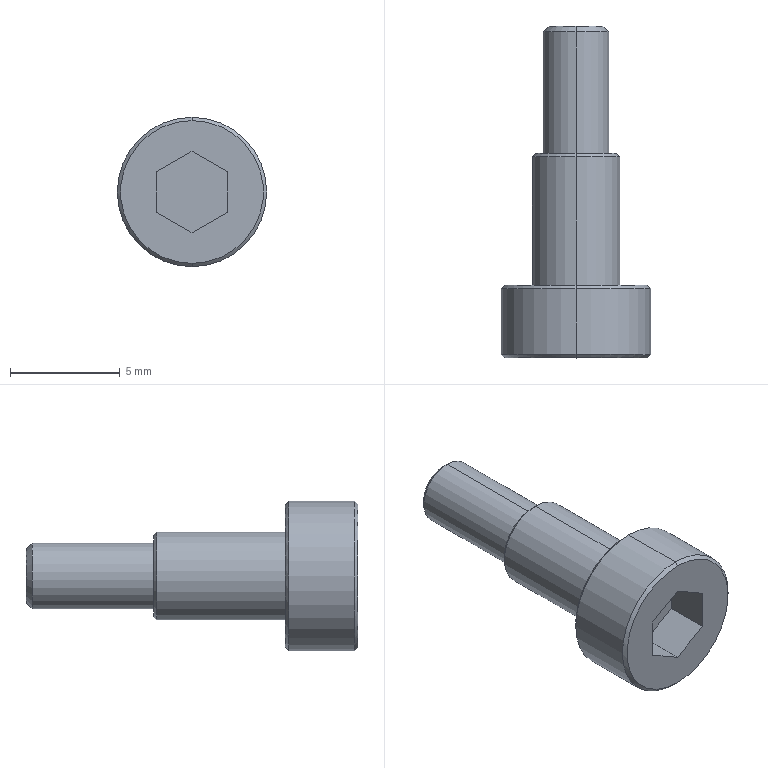Part | SolidWorks | features ICE 2, Chamfer 1, Extrusion 1, StudWizard 1 | 1 solid | 25 faces | box 6.8 x 15.1 x 6.8 mm | volume 217.57 mm3 | plane 11 | cone 8 | cylinder 6 | commonest cylinder face diameters 3 x2 4 x2 6.8 x2
STEP:
#1=CARTESIAN_POINT('',(0.,9.3,1.85));
#2=VERTEX_POINT('',#1);
#3=CARTESIAN_POINT('',(0.,9.3,-1.85));
#4=VERTEX_POINT('',#3);
#5=CARTESIAN_POINT('',(0.,9.3,0.));
#6=DIRECTION('',(0.,1.,0.));
#7=DIRECTION('',(0.,0.,1.));
#8=AXIS2_PLACEMENT_3D('',#5,#6,#7);
#9=CIRCLE('',#8,1.85);
#10=EDGE_CURVE('',#2,#4,#9,.T.);
#11=ORIENTED_EDGE('',*,*,#10,.F.);
#12=CARTESIAN_POINT('',(0.,9.15,2.));
#13=VERTEX_POINT('',#12);
#14=CARTESIAN_POINT('',(0.,9.3,1.85));
#15=DIRECTION('',(0.,-0.7071,0.7071));
#16=VECTOR('',#15,1000.);
#17=LINE('',#14,#16);
#18=EDGE_CURVE('',#2,#13,#17,.T.);
#19=ORIENTED_EDGE('',*,*,#18,.T.);
#20=CARTESIAN_POINT('',(0.,9.15,-2.));
#21=VERTEX_POINT('',#20);
#22=CARTESIAN_POINT('',(0.,9.15,0.));
#23=DIRECTION('',(0.,-1.,0.));
#24=DIRECTION('',(0.,0.,1.));
#25=AXIS2_PLACEMENT_3D('',#22,#23,#24);
#26=CIRCLE('',#25,2.);
#27=EDGE_CURVE('',#21,#13,#26,.T.);
#28=ORIENTED_EDGE('',*,*,#27,.F.);
#29=CARTESIAN_POINT('',(0.,9.3,-1.85));
#30=DIRECTION('',(0.,-0.7071,-0.7071));
#31=VECTOR('',#30,1000.);
#32=LINE('',#29,#31);
#33=EDGE_CURVE('',#4,#21,#32,.T.);
#34=ORIENTED_EDGE('',*,*,#33,.F.);
#35=EDGE_LOOP('',(#11,#19,#28,#34));
#36=FACE_OUTER_BOUND('',#35,.T.);
#37=CARTESIAN_POINT('',(0.,9.3,0.));
#38=DIRECTION('',(0.,-1.,0.));
#39=DIRECTION('',(0.,0.,-1.));
#40=AXIS2_PLACEMENT_3D('',#37,#38,#39);
#41=CONICAL_SURFACE('',#40,1.85,0.7854);
#42=ADVANCED_FACE('',(#36),#41,.T.);
#43=CARTESIAN_POINT('',(0.,3.3,3.25));
#44=VERTEX_POINT('',#43);
#45=CARTESIAN_POINT('',(0.,3.3,-3.25));
#46=VERTEX_POINT('',#45);
#47=CARTESIAN_POINT('',(0.,3.3,0.));
#48=DIRECTION('',(0.,1.,0.));
#49=DIRECTION('',(0.,0.,1.));
#50=AXIS2_PLACEMENT_3D('',#47,#48,#49);
#51=CIRCLE('',#50,3.25);
#52=EDGE_CURVE('',#44,#46,#51,.T.);
#53=ORIENTED_EDGE('',*,*,#52,.F.);
#54=CARTESIAN_POINT('',(0.,3.15,3.4));
#55=VERTEX_POINT('',#54);
#56=CARTESIAN_POINT('',(0.,3.3,3.25));
#57=DIRECTION('',(0.,-0.7071,0.7071));
#58=VECTOR('',#57,1000.);
#59=LINE('',#56,#58);
#60=EDGE_CURVE('',#44,#55,#59,.T.);
#61=ORIENTED_EDGE('',*,*,#60,.T.);
#62=CARTESIAN_POINT('',(0.,3.15,-3.4));
#63=VERTEX_POINT('',#62);
#64=CARTESIAN_POINT('',(0.,3.15,0.));
#65=DIRECTION('',(0.,-1.,0.));
#66=DIRECTION('',(0.,0.,1.));
#67=AXIS2_PLACEMENT_3D('',#64,#65,#66);
#68=CIRCLE('',#67,3.4);
#69=EDGE_CURVE('',#63,#55,#68,.T.);
#70=ORIENTED_EDGE('',*,*,#69,.F.);
#71=CARTESIAN_POINT('',(0.,3.3,-3.25));
#72=DIRECTION('',(0.,-0.7071,-0.7071));
#73=VECTOR('',#72,1000.);
#74=LINE('',#71,#73);
#75=EDGE_CURVE('',#46,#63,#74,.T.);
#76=ORIENTED_EDGE('',*,*,#75,.F.);
#77=EDGE_LOOP('',(#53,#61,#70,#76));
#78=FACE_OUTER_BOUND('',#77,.T.);
#79=CARTESIAN_POINT('',(0.,3.3,0.));
#80=DIRECTION('',(0.,-1.,0.));
#81=DIRECTION('',(0.,0.,-1.));
#82=AXIS2_PLACEMENT_3D('',#79,#80,#81);
#83=CONICAL_SURFACE('',#82,3.25,0.7854);
#84=ADVANCED_FACE('',(#78),#83,.T.);
#85=CARTESIAN_POINT('',(0.,0.,-3.25));
#86=VERTEX_POINT('',#85);
#87=CARTESIAN_POINT('',(0.,0.,3.25));
#88=VERTEX_POINT('',#87);
#89=CARTESIAN_POINT('',(0.,0.,0.));
#90=DIRECTION('',(0.,-1.,0.));
#91=DIRECTION('',(0.,0.,1.));
#92=AXIS2_PLACEMENT_3D('',#89,#90,#91);
#93=CIRCLE('',#92,3.25);
#94=EDGE_CURVE('',#86,#88,#93,.T.);
#95=ORIENTED_EDGE('',*,*,#94,.F.);
#96=CARTESIAN_POINT('',(0.,0.15,-3.4));
#97=VERTEX_POINT('',#96);
#98=CARTESIAN_POINT('',(0.,0.15,-3.4));
#99=DIRECTION('',(0.,0.7071,-0.7071));
#100=VECTOR('',#99,1000.);
#101=LINE('',#98,#100);
#102=EDGE_CURVE('',#86,#97,#101,.T.);
#103=ORIENTED_EDGE('',*,*,#102,.T.);
#104=CARTESIAN_POINT('',(0.,0.15,3.4));
#105=VERTEX_POINT('',#104);
#106=CARTESIAN_POINT('',(0.,0.15,0.));
#107=DIRECTION('',(0.,1.,0.));
#108=DIRECTION('',(0.,0.,1.));
#109=AXIS2_PLACEMENT_3D('',#106,#107,#108);
#110=CIRCLE('',#109,3.4);
#111=EDGE_CURVE('',#105,#97,#110,.T.);
#112=ORIENTED_EDGE('',*,*,#111,.F.);
#113=CARTESIAN_POINT('',(0.,0.15,3.4));
#114=DIRECTION('',(0.,0.7071,0.7071));
#115=VECTOR('',#114,1000.);
#116=LINE('',#113,#115);
#117=EDGE_CURVE('',#88,#105,#116,.T.);
#118=ORIENTED_EDGE('',*,*,#117,.F.);
#119=EDGE_LOOP('',(#95,#103,#112,#118));
#120=FACE_OUTER_BOUND('',#119,.T.);
#121=CARTESIAN_POINT('',(0.,0.15,0.));
#122=DIRECTION('',(0.,1.,0.));
#123=DIRECTION('',(0.,0.,1.));
#124=AXIS2_PLACEMENT_3D('',#121,#122,#123);
#125=CONICAL_SURFACE('',#124,3.4,0.7854);
#126=ADVANCED_FACE('',(#120),#125,.T.);
#127=CARTESIAN_POINT('',(0.,14.83,-1.5));
#128=VERTEX_POINT('',#127);
#129=CARTESIAN_POINT('',(0.,14.83,1.5));
#130=VERTEX_POINT('',#129);
#131=CARTESIAN_POINT('',(0.,14.83,0.));
#132=DIRECTION('',(0.,-1.,0.));
#133=DIRECTION('',(0.,0.,-1.));
#134=AXIS2_PLACEMENT_3D('',#131,#132,#133);
#135=CIRCLE('',#134,1.5);
#136=EDGE_CURVE('',#128,#130,#135,.T.);
#137=ORIENTED_EDGE('',*,*,#136,.T.);
#138=CARTESIAN_POINT('',(0.,9.3,1.5));
#139=VERTEX_POINT('',#138);
#140=CARTESIAN_POINT('',(0.,9.3,1.5));
#141=DIRECTION('',(0.,-1.,0.));
#142=VECTOR('',#141,1000.);
#143=LINE('',#140,#142);
#144=EDGE_CURVE('',#130,#139,#143,.T.);
#145=ORIENTED_EDGE('',*,*,#144,.T.);
#146=CARTESIAN_POINT('',(0.,9.3,-1.5));
#147=VERTEX_POINT('',#146);
#148=CARTESIAN_POINT('',(0.,9.3,0.));
#149=DIRECTION('',(0.,-1.,0.));
#150=DIRECTION('',(0.,0.,-1.));
#151=AXIS2_PLACEMENT_3D('',#148,#149,#150);
#152=CIRCLE('',#151,1.5);
#153=EDGE_CURVE('',#147,#139,#152,.T.);
#154=ORIENTED_EDGE('',*,*,#153,.F.);
#155=CARTESIAN_POINT('',(0.,9.3,-1.5));
#156=DIRECTION('',(0.,-1.,0.));
#157=VECTOR('',#156,1000.);
#158=LINE('',#155,#157);
#159=EDGE_CURVE('',#128,#147,#158,.T.);
#160=ORIENTED_EDGE('',*,*,#159,.F.);
#161=EDGE_LOOP('',(#137,#145,#154,#160));
#162=FACE_OUTER_BOUND('',#161,.T.);
#163=CARTESIAN_POINT('',(0.,9.3,0.));
#164=DIRECTION('',(0.,-1.,0.));
#165=DIRECTION('',(0.,0.,-1.));
#166=AXIS2_PLACEMENT_3D('',#163,#164,#165);
#167=CYLINDRICAL_SURFACE('',#166,1.5);
#168=ADVANCED_FACE('',(#162),#167,.T.);
#169=CARTESIAN_POINT('',(0.,15.1,-1.23));
#170=VERTEX_POINT('',#169);
#171=CARTESIAN_POINT('',(0.,15.1,1.23));
#172=VERTEX_POINT('',#171);
#173=CARTESIAN_POINT('',(0.,15.1,0.));
#174=DIRECTION('',(0.,-1.,0.));
#175=DIRECTION('',(0.,0.,-1.));
#176=AXIS2_PLACEMENT_3D('',#173,#174,#175);
#177=CIRCLE('',#176,1.23);
#178=EDGE_CURVE('',#170,#172,#177,.T.);
#179=ORIENTED_EDGE('',*,*,#178,.T.);
#180=CARTESIAN_POINT('',(0.,14.83,1.5));
#181=DIRECTION('',(0.,-0.7071,0.7071));
#182=VECTOR('',#181,1000.);
#183=LINE('',#180,#182);
#184=EDGE_CURVE('',#172,#130,#183,.T.);
#185=ORIENTED_EDGE('',*,*,#184,.T.);
#186=ORIENTED_EDGE('',*,*,#136,.F.);
#187=CARTESIAN_POINT('',(0.,14.83,-1.5));
#188=DIRECTION('',(0.,-0.7071,-0.7071));
#189=VECTOR('',#188,1000.);
#190=LINE('',#187,#189);
#191=EDGE_CURVE('',#170,#128,#190,.T.);
#192=ORIENTED_EDGE('',*,*,#191,.F.);
#193=EDGE_LOOP('',(#179,#185,#186,#192));
#194=FACE_OUTER_BOUND('',#193,.T.);
#195=CARTESIAN_POINT('',(0.,14.83,0.));
#196=DIRECTION('',(0.,-1.,0.));
#197=DIRECTION('',(0.,0.,-1.));
#198=AXIS2_PLACEMENT_3D('',#195,#196,#197);
#199=CONICAL_SURFACE('',#198,1.5,0.7854);
#200=ADVANCED_FACE('',(#194),#199,.T.);
#201=ORIENTED_EDGE('',*,*,#27,.T.);
#202=CARTESIAN_POINT('',(0.,3.3,2.));
#203=VERTEX_POINT('',#202);
#204=CARTESIAN_POINT('',(0.,9.3,2.));
#205=DIRECTION('',(0.,-1.,0.));
#206=VECTOR('',#205,1000.);
#207=LINE('',#204,#206);
#208=EDGE_CURVE('',#13,#203,#207,.T.);
#209=ORIENTED_EDGE('',*,*,#208,.T.);
#210=CARTESIAN_POINT('',(0.,3.3,-2.));
#211=VERTEX_POINT('',#210);
#212=CARTESIAN_POINT('',(0.,3.3,0.));
#213=DIRECTION('',(0.,1.,0.));
#214=DIRECTION('',(0.,0.,1.));
#215=AXIS2_PLACEMENT_3D('',#212,#213,#214);
#216=CIRCLE('',#215,2.);
#217=EDGE_CURVE('',#203,#211,#216,.T.);
#218=ORIENTED_EDGE('',*,*,#217,.T.);
#219=CARTESIAN_POINT('',(0.,9.3,-2.));
#220=DIRECTION('',(0.,-1.,0.));
#221=VECTOR('',#220,1000.);
#222=LINE('',#219,#221);
#223=EDGE_CURVE('',#21,#211,#222,.T.);
#224=ORIENTED_EDGE('',*,*,#223,.F.);
#225=EDGE_LOOP('',(#201,#209,#218,#224));
#226=FACE_OUTER_BOUND('',#225,.T.);
#227=CARTESIAN_POINT('',(0.,9.3,0.));
#228=DIRECTION('',(0.,-1.,0.));
#229=DIRECTION('',(0.,0.,-1.));
#230=AXIS2_PLACEMENT_3D('',#227,#228,#229);
#231=CYLINDRICAL_SURFACE('',#230,2.);
#232=ADVANCED_FACE('',(#226),#231,.T.);
#233=ORIENTED_EDGE('',*,*,#69,.T.);
#234=CARTESIAN_POINT('',(0.,3.3,3.4));
#235=DIRECTION('',(0.,-1.,0.));
#236=VECTOR('',#235,1000.);
#237=LINE('',#234,#236);
#238=EDGE_CURVE('',#55,#105,#237,.T.);
#239=ORIENTED_EDGE('',*,*,#238,.T.);
#240=ORIENTED_EDGE('',*,*,#111,.T.);
#241=CARTESIAN_POINT('',(0.,3.3,-3.4));
#242=DIRECTION('',(0.,-1.,0.));
#243=VECTOR('',#242,1000.);
#244=LINE('',#241,#243);
#245=EDGE_CURVE('',#63,#97,#244,.T.);
#246=ORIENTED_EDGE('',*,*,#245,.F.);
#247=EDGE_LOOP('',(#233,#239,#240,#246));
#248=FACE_OUTER_BOUND('',#247,.T.);
#249=CARTESIAN_POINT('',(0.,3.3,0.));
#250=DIRECTION('',(0.,-1.,0.));
#251=DIRECTION('',(0.,0.,-1.));
#252=AXIS2_PLACEMENT_3D('',#249,#250,#251);
#253=CYLINDRICAL_SURFACE('',#252,3.4);
#254=ADVANCED_FACE('',(#248),#253,.T.);
#255=ORIENTED_EDGE('',*,*,#238,.F.);
#256=CARTESIAN_POINT('',(0.,3.15,0.));
#257=DIRECTION('',(0.,-1.,0.));
#258=DIRECTION('',(0.,0.,1.));
#259=AXIS2_PLACEMENT_3D('',#256,#257,#258);
#260=CIRCLE('',#259,3.4);
#261=EDGE_CURVE('',#55,#63,#260,.T.);
#262=ORIENTED_EDGE('',*,*,#261,.T.);
#263=ORIENTED_EDGE('',*,*,#245,.T.);
#264=CARTESIAN_POINT('',(0.,0.15,0.));
#265=DIRECTION('',(0.,1.,0.));
#266=DIRECTION('',(0.,0.,1.));
#267=AXIS2_PLACEMENT_3D('',#264,#265,#266);
#268=CIRCLE('',#267,3.4);
#269=EDGE_CURVE('',#97,#105,#268,.T.);
#270=ORIENTED_EDGE('',*,*,#269,.T.);
#271=EDGE_LOOP('',(#255,#262,#263,#270));
#272=FACE_OUTER_BOUND('',#271,.T.);
#273=CARTESIAN_POINT('',(0.,3.3,0.));
#274=DIRECTION('',(0.,-1.,0.));
#275=DIRECTION('',(0.,0.,-1.));
#276=AXIS2_PLACEMENT_3D('',#273,#274,#275);
#277=CYLINDRICAL_SURFACE('',#276,3.4);
#278=ADVANCED_FACE('',(#272),#277,.T.);
#279=CARTESIAN_POINT('',(0.,3.3,0.));
#280=DIRECTION('',(0.,1.,0.));
#281=DIRECTION('',(0.,0.,1.));
#282=AXIS2_PLACEMENT_3D('',#279,#280,#281);
#283=CIRCLE('',#282,3.25);
#284=EDGE_CURVE('',#46,#44,#283,.T.);
#285=ORIENTED_EDGE('',*,*,#284,.T.);
#286=ORIENTED_EDGE('',*,*,#52,.T.);
#287=EDGE_LOOP('',(#285,#286));
#288=FACE_OUTER_BOUND('',#287,.T.);
#289=CARTESIAN_POINT('',(0.,3.3,0.));
#290=DIRECTION('',(0.,1.,0.));
#291=DIRECTION('',(0.,0.,1.));
#292=AXIS2_PLACEMENT_3D('',#289,#290,#291);
#293=CIRCLE('',#292,2.);
#294=EDGE_CURVE('',#211,#203,#293,.T.);
#295=ORIENTED_EDGE('',*,*,#294,.F.);
#296=ORIENTED_EDGE('',*,*,#217,.F.);
#297=EDGE_LOOP('',(#295,#296));
#298=FACE_BOUND('',#297,.T.);
#299=CARTESIAN_POINT('',(0.,3.3,0.));
#300=DIRECTION('',(0.,1.,0.));
#301=DIRECTION('',(0.,0.,1.));
#302=AXIS2_PLACEMENT_3D('',#299,#300,#301);
#303=PLANE('',#302);
#304=ADVANCED_FACE('',(#288,#298),#303,.T.);
#305=CARTESIAN_POINT('',(0.,0.,0.));
#306=DIRECTION('',(0.,-1.,0.));
#307=DIRECTION('',(0.,0.,1.));
#308=AXIS2_PLACEMENT_3D('',#305,#306,#307);
#309=CIRCLE('',#308,3.25);
#310=EDGE_CURVE('',#88,#86,#309,.T.);
#311=ORIENTED_EDGE('',*,*,#310,.T.);
#312=ORIENTED_EDGE('',*,*,#94,.T.);
#313=EDGE_LOOP('',(#311,#312));
#314=FACE_OUTER_BOUND('',#313,.T.);
#315=CARTESIAN_POINT('',(0.,0.,1.848));
#316=VERTEX_POINT('',#315);
#317=CARTESIAN_POINT('',(-1.6,0.,0.9238));
#318=VERTEX_POINT('',#317);
#319=CARTESIAN_POINT('',(0.,0.,1.848));
#320=DIRECTION('',(-0.866,0.,-0.5));
#321=VECTOR('',#320,1000.);
#322=LINE('',#319,#321);
#323=EDGE_CURVE('',#316,#318,#322,.T.);
#324=ORIENTED_EDGE('',*,*,#323,.F.);
#325=CARTESIAN_POINT('',(1.6,0.,0.9238));
#326=VERTEX_POINT('',#325);
#327=CARTESIAN_POINT('',(1.6,0.,0.9238));
#328=DIRECTION('',(-0.866,0.,0.5));
#329=VECTOR('',#328,1000.);
#330=LINE('',#327,#329);
#331=EDGE_CURVE('',#326,#316,#330,.T.);
#332=ORIENTED_EDGE('',*,*,#331,.F.);
#333=CARTESIAN_POINT('',(1.6,0.,-0.9238));
#334=VERTEX_POINT('',#333);
#335=CARTESIAN_POINT('',(1.6,0.,-0.9238));
#336=DIRECTION('',(0.,0.,1.));
#337=VECTOR('',#336,1000.);
#338=LINE('',#335,#337);
#339=EDGE_CURVE('',#334,#326,#338,.T.);
#340=ORIENTED_EDGE('',*,*,#339,.F.);
#341=CARTESIAN_POINT('',(0.,0.,-1.848));
#342=VERTEX_POINT('',#341);
#343=CARTESIAN_POINT('',(0.,0.,-1.848));
#344=DIRECTION('',(0.866,0.,0.5));
#345=VECTOR('',#344,1000.);
#346=LINE('',#343,#345);
#347=EDGE_CURVE('',#342,#334,#346,.T.);
#348=ORIENTED_EDGE('',*,*,#347,.F.);
#349=CARTESIAN_POINT('',(-1.6,0.,-0.9238));
#350=VERTEX_POINT('',#349);
#351=CARTESIAN_POINT('',(-1.6,0.,-0.9238));
#352=DIRECTION('',(0.866,0.,-0.5));
#353=VECTOR('',#352,1000.);
#354=LINE('',#351,#353);
#355=EDGE_CURVE('',#350,#342,#354,.T.);
#356=ORIENTED_EDGE('',*,*,#355,.F.);
#357=CARTESIAN_POINT('',(-1.6,0.,0.9238));
#358=DIRECTION('',(0.,0.,-1.));
#359=VECTOR('',#358,1000.);
#360=LINE('',#357,#359);
#361=EDGE_CURVE('',#318,#350,#360,.T.);
#362=ORIENTED_EDGE('',*,*,#361,.F.);
#363=EDGE_LOOP('',(#324,#332,#340,#348,#356,#362));
#364=FACE_BOUND('',#363,.T.);
#365=CARTESIAN_POINT('',(0.,0.,0.));
#366=DIRECTION('',(0.,1.,0.));
#367=DIRECTION('',(0.,0.,1.));
#368=AXIS2_PLACEMENT_3D('',#365,#366,#367);
#369=PLANE('',#368);
#370=ADVANCED_FACE('',(#314,#364),#369,.F.);
#371=ORIENTED_EDGE('',*,*,#208,.F.);
#372=CARTESIAN_POINT('',(0.,9.15,0.));
#373=DIRECTION('',(0.,-1.,0.));
#374=DIRECTION('',(0.,0.,1.));
#375=AXIS2_PLACEMENT_3D('',#372,#373,#374);
#376=CIRCLE('',#375,2.);
#377=EDGE_CURVE('',#13,#21,#376,.T.);
#378=ORIENTED_EDGE('',*,*,#377,.T.);
#379=ORIENTED_EDGE('',*,*,#223,.T.);
#380=ORIENTED_EDGE('',*,*,#294,.T.);
#381=EDGE_LOOP('',(#371,#378,#379,#380));
#382=FACE_OUTER_BOUND('',#381,.T.);
#383=CARTESIAN_POINT('',(0.,9.3,0.));
#384=DIRECTION('',(0.,-1.,0.));
#385=DIRECTION('',(0.,0.,-1.));
#386=AXIS2_PLACEMENT_3D('',#383,#384,#385);
#387=CYLINDRICAL_SURFACE('',#386,2.);
#388=ADVANCED_FACE('',(#382),#387,.T.);
#389=CARTESIAN_POINT('',(0.,9.3,0.));
#390=DIRECTION('',(0.,1.,0.));
#391=DIRECTION('',(0.,0.,1.));
#392=AXIS2_PLACEMENT_3D('',#389,#390,#391);
#393=CIRCLE('',#392,1.85);
#394=EDGE_CURVE('',#4,#2,#393,.T.);
#395=ORIENTED_EDGE('',*,*,#394,.T.);
#396=ORIENTED_EDGE('',*,*,#10,.T.);
#397=EDGE_LOOP('',(#395,#396));
#398=FACE_OUTER_BOUND('',#397,.T.);
#399=ORIENTED_EDGE('',*,*,#153,.T.);
#400=CARTESIAN_POINT('',(0.,9.3,0.));
#401=DIRECTION('',(0.,-1.,0.));
#402=DIRECTION('',(0.,0.,-1.));
#403=AXIS2_PLACEMENT_3D('',#400,#401,#402);
#404=CIRCLE('',#403,1.5);
#405=EDGE_CURVE('',#139,#147,#404,.T.);
#406=ORIENTED_EDGE('',*,*,#405,.T.);
#407=EDGE_LOOP('',(#399,#406));
#408=FACE_BOUND('',#407,.T.);
#409=CARTESIAN_POINT('',(0.,9.3,0.));
#410=DIRECTION('',(0.,1.,0.));
#411=DIRECTION('',(0.,0.,1.));
#412=AXIS2_PLACEMENT_3D('',#409,#410,#411);
#413=PLANE('',#412);
#414=ADVANCED_FACE('',(#398,#408),#413,.T.);
#415=ORIENTED_EDGE('',*,*,#178,.F.);
#416=CARTESIAN_POINT('',(0.,15.1,0.));
#417=DIRECTION('',(0.,-1.,0.));
#418=DIRECTION('',(0.,0.,-1.));
#419=AXIS2_PLACEMENT_3D('',#416,#417,#418);
#420=CIRCLE('',#419,1.23);
#421=EDGE_CURVE('',#172,#170,#420,.T.);
#422=ORIENTED_EDGE('',*,*,#421,.F.);
#423=EDGE_LOOP('',(#415,#422));
#424=FACE_OUTER_BOUND('',#423,.T.);
#425=CARTESIAN_POINT('',(1.23,15.1,0.));
#426=DIRECTION('',(0.,1.,0.));
#427=DIRECTION('',(0.,0.,1.));
#428=AXIS2_PLACEMENT_3D('',#425,#426,#427);
#429=PLANE('',#428);
#430=ADVANCED_FACE('',(#424),#429,.T.);
#431=ORIENTED_EDGE('',*,*,#184,.F.);
#432=ORIENTED_EDGE('',*,*,#421,.T.);
#433=ORIENTED_EDGE('',*,*,#191,.T.);
#434=CARTESIAN_POINT('',(0.,14.83,0.));
#435=DIRECTION('',(0.,-1.,0.));
#436=DIRECTION('',(0.,0.,-1.));
#437=AXIS2_PLACEMENT_3D('',#434,#435,#436);
#438=CIRCLE('',#437,1.5);
#439=EDGE_CURVE('',#130,#128,#438,.T.);
#440=ORIENTED_EDGE('',*,*,#439,.F.);
#441=EDGE_LOOP('',(#431,#432,#433,#440));
#442=FACE_OUTER_BOUND('',#441,.T.);
#443=CARTESIAN_POINT('',(0.,14.83,0.));
#444=DIRECTION('',(0.,-1.,0.));
#445=DIRECTION('',(0.,0.,-1.));
#446=AXIS2_PLACEMENT_3D('',#443,#444,#445);
#447=CONICAL_SURFACE('',#446,1.5,0.7854);
#448=ADVANCED_FACE('',(#442),#447,.T.);
#449=ORIENTED_EDGE('',*,*,#144,.F.);
#450=ORIENTED_EDGE('',*,*,#439,.T.);
#451=ORIENTED_EDGE('',*,*,#159,.T.);
#452=ORIENTED_EDGE('',*,*,#405,.F.);
#453=EDGE_LOOP('',(#449,#450,#451,#452));
#454=FACE_OUTER_BOUND('',#453,.T.);
#455=CARTESIAN_POINT('',(0.,9.3,0.));
#456=DIRECTION('',(0.,-1.,0.));
#457=DIRECTION('',(0.,0.,-1.));
#458=AXIS2_PLACEMENT_3D('',#455,#456,#457);
#459=CYLINDRICAL_SURFACE('',#458,1.5);
#460=ADVANCED_FACE('',(#454),#459,.T.);
#461=ORIENTED_EDGE('',*,*,#331,.T.);
#462=CARTESIAN_POINT('',(0.,2.,1.848));
#463=VERTEX_POINT('',#462);
#464=CARTESIAN_POINT('',(0.,2.,1.848));
#465=DIRECTION('',(0.,-1.,0.));
#466=VECTOR('',#465,1000.);
#467=LINE('',#464,#466);
#468=EDGE_CURVE('',#463,#316,#467,.T.);
#469=ORIENTED_EDGE('',*,*,#468,.F.);
#470=CARTESIAN_POINT('',(1.6,2.,0.9238));
#471=VERTEX_POINT('',#470);
#472=CARTESIAN_POINT('',(1.6,2.,0.9238));
#473=DIRECTION('',(-0.866,0.,0.5));
#474=VECTOR('',#473,1000.);
#475=LINE('',#472,#474);
#476=EDGE_CURVE('',#471,#463,#475,.T.);
#477=ORIENTED_EDGE('',*,*,#476,.F.);
#478=CARTESIAN_POINT('',(1.6,2.,0.9238));
#479=DIRECTION('',(0.,-1.,0.));
#480=VECTOR('',#479,1000.);
#481=LINE('',#478,#480);
#482=EDGE_CURVE('',#471,#326,#481,.T.);
#483=ORIENTED_EDGE('',*,*,#482,.T.);
#484=EDGE_LOOP('',(#461,#469,#477,#483));
#485=FACE_OUTER_BOUND('',#484,.T.);
#486=CARTESIAN_POINT('',(1.6,2.,0.9238));
#487=DIRECTION('',(0.5,0.,0.866));
#488=DIRECTION('',(0.866,0.,-0.5));
#489=AXIS2_PLACEMENT_3D('',#486,#487,#488);
#490=PLANE('',#489);
#491=ADVANCED_FACE('',(#485),#490,.F.);
#492=ORIENTED_EDGE('',*,*,#339,.T.);
#493=ORIENTED_EDGE('',*,*,#482,.F.);
#494=CARTESIAN_POINT('',(1.6,2.,-0.9238));
#495=VERTEX_POINT('',#494);
#496=CARTESIAN_POINT('',(1.6,2.,-0.9238));
#497=DIRECTION('',(0.,0.,1.));
#498=VECTOR('',#497,1000.);
#499=LINE('',#496,#498);
#500=EDGE_CURVE('',#495,#471,#499,.T.);
#501=ORIENTED_EDGE('',*,*,#500,.F.);
#502=CARTESIAN_POINT('',(1.6,2.,-0.9238));
#503=DIRECTION('',(0.,-1.,0.));
#504=VECTOR('',#503,1000.);
#505=LINE('',#502,#504);
#506=EDGE_CURVE('',#495,#334,#505,.T.);
#507=ORIENTED_EDGE('',*,*,#506,.T.);
#508=EDGE_LOOP('',(#492,#493,#501,#507));
#509=FACE_OUTER_BOUND('',#508,.T.);
#510=CARTESIAN_POINT('',(1.6,2.,-0.9238));
#511=DIRECTION('',(1.,0.,0.));
#512=DIRECTION('',(0.,0.,-1.));
#513=AXIS2_PLACEMENT_3D('',#510,#511,#512);
#514=PLANE('',#513);
#515=ADVANCED_FACE('',(#509),#514,.F.);
#516=ORIENTED_EDGE('',*,*,#347,.T.);
#517=ORIENTED_EDGE('',*,*,#506,.F.);
#518=CARTESIAN_POINT('',(0.,2.,-1.848));
#519=VERTEX_POINT('',#518);
#520=CARTESIAN_POINT('',(0.,2.,-1.848));
#521=DIRECTION('',(0.866,0.,0.5));
#522=VECTOR('',#521,1000.);
#523=LINE('',#520,#522);
#524=EDGE_CURVE('',#519,#495,#523,.T.);
#525=ORIENTED_EDGE('',*,*,#524,.F.);
#526=CARTESIAN_POINT('',(0.,2.,-1.848));
#527=DIRECTION('',(0.,-1.,0.));
#528=VECTOR('',#527,1000.);
#529=LINE('',#526,#528);
#530=EDGE_CURVE('',#519,#342,#529,.T.);
#531=ORIENTED_EDGE('',*,*,#530,.T.);
#532=EDGE_LOOP('',(#516,#517,#525,#531));
#533=FACE_OUTER_BOUND('',#532,.T.);
#534=CARTESIAN_POINT('',(0.,2.,-1.848));
#535=DIRECTION('',(0.5,0.,-0.866));
#536=DIRECTION('',(-0.866,0.,-0.5));
#537=AXIS2_PLACEMENT_3D('',#534,#535,#536);
#538=PLANE('',#537);
#539=ADVANCED_FACE('',(#533),#538,.F.);
#540=ORIENTED_EDGE('',*,*,#355,.T.);
#541=ORIENTED_EDGE('',*,*,#530,.F.);
#542=CARTESIAN_POINT('',(-1.6,2.,-0.9238));
#543=VERTEX_POINT('',#542);
#544=CARTESIAN_POINT('',(-1.6,2.,-0.9238));
#545=DIRECTION('',(0.866,0.,-0.5));
#546=VECTOR('',#545,1000.);
#547=LINE('',#544,#546);
#548=EDGE_CURVE('',#543,#519,#547,.T.);
#549=ORIENTED_EDGE('',*,*,#548,.F.);
#550=CARTESIAN_POINT('',(-1.6,2.,-0.9238));
#551=DIRECTION('',(0.,-1.,0.));
#552=VECTOR('',#551,1000.);
#553=LINE('',#550,#552);
#554=EDGE_CURVE('',#543,#350,#553,.T.);
#555=ORIENTED_EDGE('',*,*,#554,.T.);
#556=EDGE_LOOP('',(#540,#541,#549,#555));
#557=FACE_OUTER_BOUND('',#556,.T.);
#558=CARTESIAN_POINT('',(-1.6,2.,-0.9238));
#559=DIRECTION('',(-0.5,0.,-0.866));
#560=DIRECTION('',(-0.866,0.,0.5));
#561=AXIS2_PLACEMENT_3D('',#558,#559,#560);
#562=PLANE('',#561);
#563=ADVANCED_FACE('',(#557),#562,.F.);
#564=ORIENTED_EDGE('',*,*,#361,.T.);
#565=ORIENTED_EDGE('',*,*,#554,.F.);
#566=CARTESIAN_POINT('',(-1.6,2.,0.9238));
#567=VERTEX_POINT('',#566);
#568=CARTESIAN_POINT('',(-1.6,2.,0.9238));
#569=DIRECTION('',(0.,0.,-1.));
#570=VECTOR('',#569,1000.);
#571=LINE('',#568,#570);
#572=EDGE_CURVE('',#567,#543,#571,.T.);
#573=ORIENTED_EDGE('',*,*,#572,.F.);
#574=CARTESIAN_POINT('',(-1.6,2.,0.9238));
#575=DIRECTION('',(0.,-1.,0.));
#576=VECTOR('',#575,1000.);
#577=LINE('',#574,#576);
#578=EDGE_CURVE('',#567,#318,#577,.T.);
#579=ORIENTED_EDGE('',*,*,#578,.T.);
#580=EDGE_LOOP('',(#564,#565,#573,#579));
#581=FACE_OUTER_BOUND('',#580,.T.);
#582=CARTESIAN_POINT('',(-1.6,2.,0.9238));
#583=DIRECTION('',(-1.,0.,0.));
#584=DIRECTION('',(0.,0.,1.));
#585=AXIS2_PLACEMENT_3D('',#582,#583,#584);
#586=PLANE('',#585);
#587=ADVANCED_FACE('',(#581),#586,.F.);
#588=ORIENTED_EDGE('',*,*,#323,.T.);
#589=ORIENTED_EDGE('',*,*,#578,.F.);
#590=CARTESIAN_POINT('',(0.,2.,1.848));
#591=DIRECTION('',(-0.866,0.,-0.5));
#592=VECTOR('',#591,1000.);
#593=LINE('',#590,#592);
#594=EDGE_CURVE('',#463,#567,#593,.T.);
#595=ORIENTED_EDGE('',*,*,#594,.F.);
#596=ORIENTED_EDGE('',*,*,#468,.T.);
#597=EDGE_LOOP('',(#588,#589,#595,#596));
#598=FACE_OUTER_BOUND('',#597,.T.);
#599=CARTESIAN_POINT('',(0.,2.,1.848));
#600=DIRECTION('',(-0.5,0.,0.866));
#601=DIRECTION('',(0.866,0.,0.5));
#602=AXIS2_PLACEMENT_3D('',#599,#600,#601);
#603=PLANE('',#602);
#604=ADVANCED_FACE('',(#598),#603,.F.);
#605=ORIENTED_EDGE('',*,*,#476,.T.);
#606=ORIENTED_EDGE('',*,*,#594,.T.);
#607=ORIENTED_EDGE('',*,*,#572,.T.);
#608=ORIENTED_EDGE('',*,*,#548,.T.);
#609=ORIENTED_EDGE('',*,*,#524,.T.);
#610=ORIENTED_EDGE('',*,*,#500,.T.);
#611=EDGE_LOOP('',(#605,#606,#607,#608,#609,#610));
#612=FACE_OUTER_BOUND('',#611,.T.);
#613=CARTESIAN_POINT('',(0.,2.,0.));
#614=DIRECTION('',(0.,-1.,0.));
#615=DIRECTION('',(0.,0.,-1.));
#616=AXIS2_PLACEMENT_3D('',#613,#614,#615);
#617=PLANE('',#616);
#618=ADVANCED_FACE('',(#612),#617,.T.);
#619=ORIENTED_EDGE('',*,*,#102,.F.);
#620=ORIENTED_EDGE('',*,*,#310,.F.);
#621=ORIENTED_EDGE('',*,*,#117,.T.);
#622=ORIENTED_EDGE('',*,*,#269,.F.);
#623=EDGE_LOOP('',(#619,#620,#621,#622));
#624=FACE_OUTER_BOUND('',#623,.T.);
#625=CARTESIAN_POINT('',(0.,0.15,0.));
#626=DIRECTION('',(0.,1.,0.));
#627=DIRECTION('',(0.,0.,1.));
#628=AXIS2_PLACEMENT_3D('',#625,#626,#627);
#629=CONICAL_SURFACE('',#628,3.4,0.7854);
#630=ADVANCED_FACE('',(#624),#629,.T.);
#631=ORIENTED_EDGE('',*,*,#60,.F.);
#632=ORIENTED_EDGE('',*,*,#284,.F.);
#633=ORIENTED_EDGE('',*,*,#75,.T.);
#634=ORIENTED_EDGE('',*,*,#261,.F.);
#635=EDGE_LOOP('',(#631,#632,#633,#634));
#636=FACE_OUTER_BOUND('',#635,.T.);
#637=CARTESIAN_POINT('',(0.,3.3,0.));
#638=DIRECTION('',(0.,-1.,0.));
#639=DIRECTION('',(0.,0.,-1.));
#640=AXIS2_PLACEMENT_3D('',#637,#638,#639);
#641=CONICAL_SURFACE('',#640,3.25,0.7854);
#642=ADVANCED_FACE('',(#636),#641,.T.);
#643=ORIENTED_EDGE('',*,*,#18,.F.);
#644=ORIENTED_EDGE('',*,*,#394,.F.);
#645=ORIENTED_EDGE('',*,*,#33,.T.);
#646=ORIENTED_EDGE('',*,*,#377,.F.);
#647=EDGE_LOOP('',(#643,#644,#645,#646));
#648=FACE_OUTER_BOUND('',#647,.T.);
#649=CARTESIAN_POINT('',(0.,9.3,0.));
#650=DIRECTION('',(0.,-1.,0.));
#651=DIRECTION('',(0.,0.,-1.));
#652=AXIS2_PLACEMENT_3D('',#649,#650,#651);
#653=CONICAL_SURFACE('',#652,1.85,0.7854);
#654=ADVANCED_FACE('',(#648),#653,.T.);
#655=CLOSED_SHELL('',(#42,#84,#126,#168,#200,#232,#254,#278,#304,#370,#388,#414,#430,#448,#460,#491,#515,#539,#563,#587,#604,#618,#630,#642,#654));
#656=MANIFOLD_SOLID_BREP('',#655);
#657=CARTESIAN_POINT('',(0.,0.,0.));
#658=DIRECTION('',(0.,0.,1.));
#659=DIRECTION('',(1.,0.,0.));
#660=AXIS2_PLACEMENT_3D('',#657,#658,#659);
#661=(LENGTH_UNIT()NAMED_UNIT(*)SI_UNIT(.MILLI.,.METRE.));
#662=UNCERTAINTY_MEASURE_WITH_UNIT(LENGTH_MEASURE(0.00001),#661,'','');
#663=(NAMED_UNIT(*)PLANE_ANGLE_UNIT()SI_UNIT($,.RADIAN.));
#664=(NAMED_UNIT(*)SI_UNIT($,.STERADIAN.)SOLID_ANGLE_UNIT());
#665=(GEOMETRIC_REPRESENTATION_CONTEXT(3)GLOBAL_UNCERTAINTY_ASSIGNED_CONTEXT((#662))GLOBAL_UNIT_ASSIGNED_CONTEXT((#661,#663,#664))REPRESENTATION_CONTEXT('',''));
#666=ADVANCED_BREP_SHAPE_REPRESENTATION('',(#656,#660),#665);